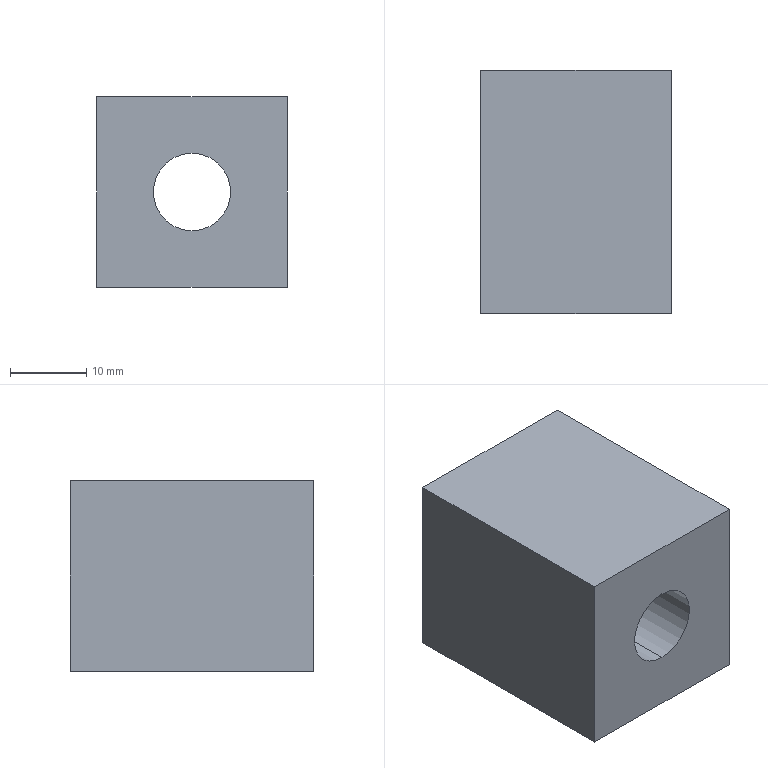Part | SolidWorks | features Extrusion 1, HoleWzd 1 | 1 solid | 8 faces | box 25 x 32 x 25 mm | volume 17385 mm3 | plane 6 | cylinder 2 | commonest cylinder face diameters 10.2 x2
STEP:
#1=CARTESIAN_POINT('',(0.,0.,-5.1));
#2=VERTEX_POINT('',#1);
#3=CARTESIAN_POINT('',(0.,0.,5.1));
#4=VERTEX_POINT('',#3);
#5=CARTESIAN_POINT('',(0.,0.,0.));
#6=DIRECTION('',(0.,1.,0.));
#7=DIRECTION('',(0.,0.,1.));
#8=AXIS2_PLACEMENT_3D('',#5,#6,#7);
#9=CIRCLE('',#8,5.1);
#10=EDGE_CURVE('',#2,#4,#9,.T.);
#11=ORIENTED_EDGE('',*,*,#10,.F.);
#12=CARTESIAN_POINT('',(0.,32.,-5.1));
#13=VERTEX_POINT('',#12);
#14=CARTESIAN_POINT('',(0.,32.,-5.1));
#15=DIRECTION('',(0.,1.,0.));
#16=VECTOR('',#15,1000.);
#17=LINE('',#14,#16);
#18=EDGE_CURVE('',#2,#13,#17,.T.);
#19=ORIENTED_EDGE('',*,*,#18,.T.);
#20=CARTESIAN_POINT('',(0.,32.,5.1));
#21=VERTEX_POINT('',#20);
#22=CARTESIAN_POINT('',(0.,32.,0.));
#23=DIRECTION('',(0.,1.,0.));
#24=DIRECTION('',(0.,0.,1.));
#25=AXIS2_PLACEMENT_3D('',#22,#23,#24);
#26=CIRCLE('',#25,5.1);
#27=EDGE_CURVE('',#13,#21,#26,.T.);
#28=ORIENTED_EDGE('',*,*,#27,.T.);
#29=CARTESIAN_POINT('',(0.,32.,5.1));
#30=DIRECTION('',(0.,1.,0.));
#31=VECTOR('',#30,1000.);
#32=LINE('',#29,#31);
#33=EDGE_CURVE('',#4,#21,#32,.T.);
#34=ORIENTED_EDGE('',*,*,#33,.F.);
#35=EDGE_LOOP('',(#11,#19,#28,#34));
#36=FACE_OUTER_BOUND('',#35,.T.);
#37=CARTESIAN_POINT('',(0.,32.,0.));
#38=DIRECTION('',(0.,1.,0.));
#39=DIRECTION('',(0.,0.,1.));
#40=AXIS2_PLACEMENT_3D('',#37,#38,#39);
#41=CYLINDRICAL_SURFACE('',#40,5.1);
#42=ADVANCED_FACE('',(#36),#41,.F.);
#43=CARTESIAN_POINT('',(12.5,0.,12.5));
#44=VERTEX_POINT('',#43);
#45=CARTESIAN_POINT('',(12.5,0.,-12.5));
#46=VERTEX_POINT('',#45);
#47=CARTESIAN_POINT('',(12.5,0.,-12.5));
#48=DIRECTION('',(0.,0.,-1.));
#49=VECTOR('',#48,1000.);
#50=LINE('',#47,#49);
#51=EDGE_CURVE('',#44,#46,#50,.T.);
#52=ORIENTED_EDGE('',*,*,#51,.T.);
#53=CARTESIAN_POINT('',(12.5,32.,-12.5));
#54=VERTEX_POINT('',#53);
#55=CARTESIAN_POINT('',(12.5,32.,-12.5));
#56=DIRECTION('',(0.,-1.,0.));
#57=VECTOR('',#56,1000.);
#58=LINE('',#55,#57);
#59=EDGE_CURVE('',#54,#46,#58,.T.);
#60=ORIENTED_EDGE('',*,*,#59,.F.);
#61=CARTESIAN_POINT('',(12.5,32.,12.5));
#62=VERTEX_POINT('',#61);
#63=CARTESIAN_POINT('',(12.5,32.,-12.5));
#64=DIRECTION('',(0.,0.,-1.));
#65=VECTOR('',#64,1000.);
#66=LINE('',#63,#65);
#67=EDGE_CURVE('',#62,#54,#66,.T.);
#68=ORIENTED_EDGE('',*,*,#67,.F.);
#69=CARTESIAN_POINT('',(12.5,32.,12.5));
#70=DIRECTION('',(0.,-1.,0.));
#71=VECTOR('',#70,1000.);
#72=LINE('',#69,#71);
#73=EDGE_CURVE('',#62,#44,#72,.T.);
#74=ORIENTED_EDGE('',*,*,#73,.T.);
#75=EDGE_LOOP('',(#52,#60,#68,#74));
#76=FACE_OUTER_BOUND('',#75,.T.);
#77=CARTESIAN_POINT('',(12.5,32.,-12.5));
#78=DIRECTION('',(-1.,0.,0.));
#79=DIRECTION('',(0.,0.,1.));
#80=AXIS2_PLACEMENT_3D('',#77,#78,#79);
#81=PLANE('',#80);
#82=ADVANCED_FACE('',(#76),#81,.F.);
#83=CARTESIAN_POINT('',(-12.5,0.,-12.5));
#84=VERTEX_POINT('',#83);
#85=CARTESIAN_POINT('',(-12.5,0.,-12.5));
#86=DIRECTION('',(-1.,0.,0.));
#87=VECTOR('',#86,1000.);
#88=LINE('',#85,#87);
#89=EDGE_CURVE('',#46,#84,#88,.T.);
#90=ORIENTED_EDGE('',*,*,#89,.T.);
#91=CARTESIAN_POINT('',(-12.5,32.,-12.5));
#92=VERTEX_POINT('',#91);
#93=CARTESIAN_POINT('',(-12.5,32.,-12.5));
#94=DIRECTION('',(0.,-1.,0.));
#95=VECTOR('',#94,1000.);
#96=LINE('',#93,#95);
#97=EDGE_CURVE('',#92,#84,#96,.T.);
#98=ORIENTED_EDGE('',*,*,#97,.F.);
#99=CARTESIAN_POINT('',(-12.5,32.,-12.5));
#100=DIRECTION('',(-1.,0.,0.));
#101=VECTOR('',#100,1000.);
#102=LINE('',#99,#101);
#103=EDGE_CURVE('',#54,#92,#102,.T.);
#104=ORIENTED_EDGE('',*,*,#103,.F.);
#105=ORIENTED_EDGE('',*,*,#59,.T.);
#106=EDGE_LOOP('',(#90,#98,#104,#105));
#107=FACE_OUTER_BOUND('',#106,.T.);
#108=CARTESIAN_POINT('',(-12.5,32.,-12.5));
#109=DIRECTION('',(0.,0.,1.));
#110=DIRECTION('',(1.,0.,0.));
#111=AXIS2_PLACEMENT_3D('',#108,#109,#110);
#112=PLANE('',#111);
#113=ADVANCED_FACE('',(#107),#112,.F.);
#114=CARTESIAN_POINT('',(-12.5,0.,12.5));
#115=VERTEX_POINT('',#114);
#116=CARTESIAN_POINT('',(-12.5,0.,-12.5));
#117=DIRECTION('',(0.,0.,1.));
#118=VECTOR('',#117,1000.);
#119=LINE('',#116,#118);
#120=EDGE_CURVE('',#84,#115,#119,.T.);
#121=ORIENTED_EDGE('',*,*,#120,.T.);
#122=CARTESIAN_POINT('',(-12.5,32.,12.5));
#123=VERTEX_POINT('',#122);
#124=CARTESIAN_POINT('',(-12.5,32.,12.5));
#125=DIRECTION('',(0.,-1.,0.));
#126=VECTOR('',#125,1000.);
#127=LINE('',#124,#126);
#128=EDGE_CURVE('',#123,#115,#127,.T.);
#129=ORIENTED_EDGE('',*,*,#128,.F.);
#130=CARTESIAN_POINT('',(-12.5,32.,-12.5));
#131=DIRECTION('',(0.,0.,1.));
#132=VECTOR('',#131,1000.);
#133=LINE('',#130,#132);
#134=EDGE_CURVE('',#92,#123,#133,.T.);
#135=ORIENTED_EDGE('',*,*,#134,.F.);
#136=ORIENTED_EDGE('',*,*,#97,.T.);
#137=EDGE_LOOP('',(#121,#129,#135,#136));
#138=FACE_OUTER_BOUND('',#137,.T.);
#139=CARTESIAN_POINT('',(-12.5,32.,-12.5));
#140=DIRECTION('',(1.,0.,0.));
#141=DIRECTION('',(0.,0.,-1.));
#142=AXIS2_PLACEMENT_3D('',#139,#140,#141);
#143=PLANE('',#142);
#144=ADVANCED_FACE('',(#138),#143,.F.);
#145=CARTESIAN_POINT('',(-12.5,0.,12.5));
#146=DIRECTION('',(1.,0.,0.));
#147=VECTOR('',#146,1000.);
#148=LINE('',#145,#147);
#149=EDGE_CURVE('',#115,#44,#148,.T.);
#150=ORIENTED_EDGE('',*,*,#149,.T.);
#151=ORIENTED_EDGE('',*,*,#73,.F.);
#152=CARTESIAN_POINT('',(-12.5,32.,12.5));
#153=DIRECTION('',(1.,0.,0.));
#154=VECTOR('',#153,1000.);
#155=LINE('',#152,#154);
#156=EDGE_CURVE('',#123,#62,#155,.T.);
#157=ORIENTED_EDGE('',*,*,#156,.F.);
#158=ORIENTED_EDGE('',*,*,#128,.T.);
#159=EDGE_LOOP('',(#150,#151,#157,#158));
#160=FACE_OUTER_BOUND('',#159,.T.);
#161=CARTESIAN_POINT('',(-12.5,32.,12.5));
#162=DIRECTION('',(0.,0.,-1.));
#163=DIRECTION('',(-1.,0.,0.));
#164=AXIS2_PLACEMENT_3D('',#161,#162,#163);
#165=PLANE('',#164);
#166=ADVANCED_FACE('',(#160),#165,.F.);
#167=CARTESIAN_POINT('',(0.,32.,0.));
#168=DIRECTION('',(0.,1.,0.));
#169=DIRECTION('',(0.,0.,1.));
#170=AXIS2_PLACEMENT_3D('',#167,#168,#169);
#171=CIRCLE('',#170,5.1);
#172=EDGE_CURVE('',#21,#13,#171,.T.);
#173=ORIENTED_EDGE('',*,*,#172,.F.);
#174=ORIENTED_EDGE('',*,*,#27,.F.);
#175=EDGE_LOOP('',(#173,#174));
#176=FACE_BOUND('',#175,.T.);
#177=ORIENTED_EDGE('',*,*,#67,.T.);
#178=ORIENTED_EDGE('',*,*,#103,.T.);
#179=ORIENTED_EDGE('',*,*,#134,.T.);
#180=ORIENTED_EDGE('',*,*,#156,.T.);
#181=EDGE_LOOP('',(#177,#178,#179,#180));
#182=FACE_OUTER_BOUND('',#181,.T.);
#183=CARTESIAN_POINT('',(0.,32.,0.));
#184=DIRECTION('',(0.,1.,0.));
#185=DIRECTION('',(0.,0.,1.));
#186=AXIS2_PLACEMENT_3D('',#183,#184,#185);
#187=PLANE('',#186);
#188=ADVANCED_FACE('',(#176,#182),#187,.T.);
#189=CARTESIAN_POINT('',(0.,0.,0.));
#190=DIRECTION('',(0.,1.,0.));
#191=DIRECTION('',(0.,0.,1.));
#192=AXIS2_PLACEMENT_3D('',#189,#190,#191);
#193=CIRCLE('',#192,5.1);
#194=EDGE_CURVE('',#4,#2,#193,.T.);
#195=ORIENTED_EDGE('',*,*,#194,.T.);
#196=ORIENTED_EDGE('',*,*,#10,.T.);
#197=EDGE_LOOP('',(#195,#196));
#198=FACE_BOUND('',#197,.T.);
#199=ORIENTED_EDGE('',*,*,#51,.F.);
#200=ORIENTED_EDGE('',*,*,#149,.F.);
#201=ORIENTED_EDGE('',*,*,#120,.F.);
#202=ORIENTED_EDGE('',*,*,#89,.F.);
#203=EDGE_LOOP('',(#199,#200,#201,#202));
#204=FACE_OUTER_BOUND('',#203,.T.);
#205=CARTESIAN_POINT('',(0.,0.,0.));
#206=DIRECTION('',(0.,1.,0.));
#207=DIRECTION('',(0.,0.,1.));
#208=AXIS2_PLACEMENT_3D('',#205,#206,#207);
#209=PLANE('',#208);
#210=ADVANCED_FACE('',(#198,#204),#209,.F.);
#211=ORIENTED_EDGE('',*,*,#18,.F.);
#212=ORIENTED_EDGE('',*,*,#194,.F.);
#213=ORIENTED_EDGE('',*,*,#33,.T.);
#214=ORIENTED_EDGE('',*,*,#172,.T.);
#215=EDGE_LOOP('',(#211,#212,#213,#214));
#216=FACE_OUTER_BOUND('',#215,.T.);
#217=CARTESIAN_POINT('',(0.,32.,0.));
#218=DIRECTION('',(0.,1.,0.));
#219=DIRECTION('',(0.,0.,1.));
#220=AXIS2_PLACEMENT_3D('',#217,#218,#219);
#221=CYLINDRICAL_SURFACE('',#220,5.1);
#222=ADVANCED_FACE('',(#216),#221,.F.);
#223=CLOSED_SHELL('',(#42,#82,#113,#144,#166,#188,#210,#222));
#224=MANIFOLD_SOLID_BREP('',#223);
#225=CARTESIAN_POINT('',(0.,0.,0.));
#226=DIRECTION('',(0.,0.,1.));
#227=DIRECTION('',(1.,0.,0.));
#228=AXIS2_PLACEMENT_3D('',#225,#226,#227);
#229=(LENGTH_UNIT()NAMED_UNIT(*)SI_UNIT(.MILLI.,.METRE.));
#230=UNCERTAINTY_MEASURE_WITH_UNIT(LENGTH_MEASURE(0.00001),#229,'','');
#231=(NAMED_UNIT(*)PLANE_ANGLE_UNIT()SI_UNIT($,.RADIAN.));
#232=(NAMED_UNIT(*)SI_UNIT($,.STERADIAN.)SOLID_ANGLE_UNIT());
#233=(GEOMETRIC_REPRESENTATION_CONTEXT(3)GLOBAL_UNCERTAINTY_ASSIGNED_CONTEXT((#230))GLOBAL_UNIT_ASSIGNED_CONTEXT((#229,#231,#232))REPRESENTATION_CONTEXT('',''));
#234=ADVANCED_BREP_SHAPE_REPRESENTATION('',(#224,#228),#233);